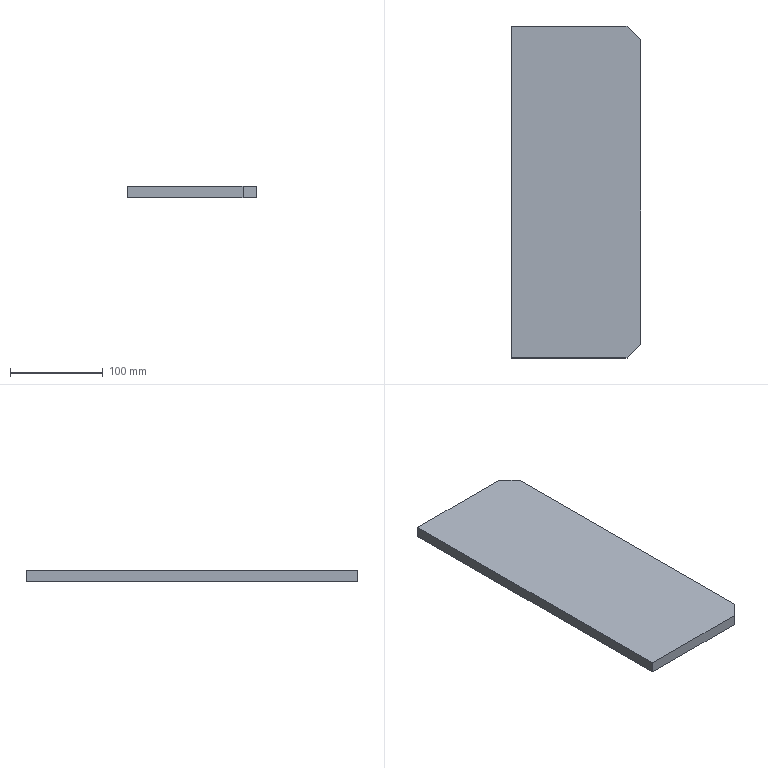Part | SolidWorks | features Chamfer 1, Extrusion 1 | 1 solid | 8 faces | box 140 x 358 x 12 mm | volume 598740 mm3 | plane 8
STEP:
#1=CARTESIAN_POINT('',(0.,358.,0.));
#2=VERTEX_POINT('',#1);
#3=CARTESIAN_POINT('',(0.,0.,0.));
#4=VERTEX_POINT('',#3);
#5=CARTESIAN_POINT('',(0.,0.,0.));
#6=DIRECTION('',(0.,-1.,0.));
#7=VECTOR('',#6,1000.);
#8=LINE('',#5,#7);
#9=EDGE_CURVE('',#2,#4,#8,.T.);
#10=ORIENTED_EDGE('',*,*,#9,.T.);
#11=CARTESIAN_POINT('',(0.,0.,12.));
#12=VERTEX_POINT('',#11);
#13=CARTESIAN_POINT('',(0.,0.,12.));
#14=DIRECTION('',(0.,0.,-1.));
#15=VECTOR('',#14,1000.);
#16=LINE('',#13,#15);
#17=EDGE_CURVE('',#12,#4,#16,.T.);
#18=ORIENTED_EDGE('',*,*,#17,.F.);
#19=CARTESIAN_POINT('',(0.,358.,12.));
#20=VERTEX_POINT('',#19);
#21=CARTESIAN_POINT('',(0.,0.,12.));
#22=DIRECTION('',(0.,-1.,0.));
#23=VECTOR('',#22,1000.);
#24=LINE('',#21,#23);
#25=EDGE_CURVE('',#20,#12,#24,.T.);
#26=ORIENTED_EDGE('',*,*,#25,.F.);
#27=CARTESIAN_POINT('',(0.,358.,12.));
#28=DIRECTION('',(0.,0.,-1.));
#29=VECTOR('',#28,1000.);
#30=LINE('',#27,#29);
#31=EDGE_CURVE('',#20,#2,#30,.T.);
#32=ORIENTED_EDGE('',*,*,#31,.T.);
#33=EDGE_LOOP('',(#10,#18,#26,#32));
#34=FACE_OUTER_BOUND('',#33,.T.);
#35=CARTESIAN_POINT('',(0.,0.,12.));
#36=DIRECTION('',(1.,0.,0.));
#37=DIRECTION('',(0.,0.,-1.));
#38=AXIS2_PLACEMENT_3D('',#35,#36,#37);
#39=PLANE('',#38);
#40=ADVANCED_FACE('',(#34),#39,.F.);
#41=CARTESIAN_POINT('',(125.,0.,0.));
#42=VERTEX_POINT('',#41);
#43=CARTESIAN_POINT('',(0.,0.,0.));
#44=DIRECTION('',(1.,0.,0.));
#45=VECTOR('',#44,1000.);
#46=LINE('',#43,#45);
#47=EDGE_CURVE('',#4,#42,#46,.T.);
#48=ORIENTED_EDGE('',*,*,#47,.T.);
#49=CARTESIAN_POINT('',(125.,0.,12.));
#50=VERTEX_POINT('',#49);
#51=CARTESIAN_POINT('',(125.,0.,12.));
#52=DIRECTION('',(0.,0.,1.));
#53=VECTOR('',#52,1000.);
#54=LINE('',#51,#53);
#55=EDGE_CURVE('',#42,#50,#54,.T.);
#56=ORIENTED_EDGE('',*,*,#55,.T.);
#57=CARTESIAN_POINT('',(0.,0.,12.));
#58=DIRECTION('',(1.,0.,0.));
#59=VECTOR('',#58,1000.);
#60=LINE('',#57,#59);
#61=EDGE_CURVE('',#12,#50,#60,.T.);
#62=ORIENTED_EDGE('',*,*,#61,.F.);
#63=ORIENTED_EDGE('',*,*,#17,.T.);
#64=EDGE_LOOP('',(#48,#56,#62,#63));
#65=FACE_OUTER_BOUND('',#64,.T.);
#66=CARTESIAN_POINT('',(0.,0.,12.));
#67=DIRECTION('',(0.,1.,0.));
#68=DIRECTION('',(0.,0.,1.));
#69=AXIS2_PLACEMENT_3D('',#66,#67,#68);
#70=PLANE('',#69);
#71=ADVANCED_FACE('',(#65),#70,.F.);
#72=CARTESIAN_POINT('',(140.,15.,12.));
#73=VERTEX_POINT('',#72);
#74=CARTESIAN_POINT('',(140.,343.,12.));
#75=VERTEX_POINT('',#74);
#76=CARTESIAN_POINT('',(140.,0.,12.));
#77=DIRECTION('',(0.,1.,0.));
#78=VECTOR('',#77,1000.);
#79=LINE('',#76,#78);
#80=EDGE_CURVE('',#73,#75,#79,.T.);
#81=ORIENTED_EDGE('',*,*,#80,.F.);
#82=CARTESIAN_POINT('',(140.,15.,0.));
#83=VERTEX_POINT('',#82);
#84=CARTESIAN_POINT('',(140.,15.,12.));
#85=DIRECTION('',(0.,0.,-1.));
#86=VECTOR('',#85,1000.);
#87=LINE('',#84,#86);
#88=EDGE_CURVE('',#73,#83,#87,.T.);
#89=ORIENTED_EDGE('',*,*,#88,.T.);
#90=CARTESIAN_POINT('',(140.,343.,0.));
#91=VERTEX_POINT('',#90);
#92=CARTESIAN_POINT('',(140.,0.,0.));
#93=DIRECTION('',(0.,1.,0.));
#94=VECTOR('',#93,1000.);
#95=LINE('',#92,#94);
#96=EDGE_CURVE('',#83,#91,#95,.T.);
#97=ORIENTED_EDGE('',*,*,#96,.T.);
#98=CARTESIAN_POINT('',(140.,343.,12.));
#99=DIRECTION('',(0.,0.,1.));
#100=VECTOR('',#99,1000.);
#101=LINE('',#98,#100);
#102=EDGE_CURVE('',#91,#75,#101,.T.);
#103=ORIENTED_EDGE('',*,*,#102,.T.);
#104=EDGE_LOOP('',(#81,#89,#97,#103));
#105=FACE_OUTER_BOUND('',#104,.T.);
#106=CARTESIAN_POINT('',(140.,0.,12.));
#107=DIRECTION('',(-1.,0.,0.));
#108=DIRECTION('',(0.,0.,1.));
#109=AXIS2_PLACEMENT_3D('',#106,#107,#108);
#110=PLANE('',#109);
#111=ADVANCED_FACE('',(#105),#110,.F.);
#112=CARTESIAN_POINT('',(125.,358.,12.));
#113=VERTEX_POINT('',#112);
#114=CARTESIAN_POINT('',(0.,358.,12.));
#115=DIRECTION('',(-1.,0.,0.));
#116=VECTOR('',#115,1000.);
#117=LINE('',#114,#116);
#118=EDGE_CURVE('',#113,#20,#117,.T.);
#119=ORIENTED_EDGE('',*,*,#118,.F.);
#120=CARTESIAN_POINT('',(125.,358.,0.));
#121=VERTEX_POINT('',#120);
#122=CARTESIAN_POINT('',(125.,358.,12.));
#123=DIRECTION('',(0.,0.,-1.));
#124=VECTOR('',#123,1000.);
#125=LINE('',#122,#124);
#126=EDGE_CURVE('',#113,#121,#125,.T.);
#127=ORIENTED_EDGE('',*,*,#126,.T.);
#128=CARTESIAN_POINT('',(0.,358.,0.));
#129=DIRECTION('',(-1.,0.,0.));
#130=VECTOR('',#129,1000.);
#131=LINE('',#128,#130);
#132=EDGE_CURVE('',#121,#2,#131,.T.);
#133=ORIENTED_EDGE('',*,*,#132,.T.);
#134=ORIENTED_EDGE('',*,*,#31,.F.);
#135=EDGE_LOOP('',(#119,#127,#133,#134));
#136=FACE_OUTER_BOUND('',#135,.T.);
#137=CARTESIAN_POINT('',(0.,358.,12.));
#138=DIRECTION('',(0.,-1.,0.));
#139=DIRECTION('',(0.,0.,-1.));
#140=AXIS2_PLACEMENT_3D('',#137,#138,#139);
#141=PLANE('',#140);
#142=ADVANCED_FACE('',(#136),#141,.F.);
#143=ORIENTED_EDGE('',*,*,#61,.T.);
#144=CARTESIAN_POINT('',(140.,15.,12.));
#145=DIRECTION('',(0.7071,0.7071,0.));
#146=VECTOR('',#145,1000.);
#147=LINE('',#144,#146);
#148=EDGE_CURVE('',#50,#73,#147,.T.);
#149=ORIENTED_EDGE('',*,*,#148,.T.);
#150=ORIENTED_EDGE('',*,*,#80,.T.);
#151=CARTESIAN_POINT('',(125.,358.,12.));
#152=DIRECTION('',(-0.7071,0.7071,0.));
#153=VECTOR('',#152,1000.);
#154=LINE('',#151,#153);
#155=EDGE_CURVE('',#75,#113,#154,.T.);
#156=ORIENTED_EDGE('',*,*,#155,.T.);
#157=ORIENTED_EDGE('',*,*,#118,.T.);
#158=ORIENTED_EDGE('',*,*,#25,.T.);
#159=EDGE_LOOP('',(#143,#149,#150,#156,#157,#158));
#160=FACE_OUTER_BOUND('',#159,.T.);
#161=CARTESIAN_POINT('',(0.,0.,12.));
#162=DIRECTION('',(0.,0.,-1.));
#163=DIRECTION('',(-1.,0.,0.));
#164=AXIS2_PLACEMENT_3D('',#161,#162,#163);
#165=PLANE('',#164);
#166=ADVANCED_FACE('',(#160),#165,.F.);
#167=ORIENTED_EDGE('',*,*,#96,.F.);
#168=CARTESIAN_POINT('',(62.5,-62.5,0.));
#169=DIRECTION('',(-0.7071,-0.7071,0.));
#170=VECTOR('',#169,1000.);
#171=LINE('',#168,#170);
#172=EDGE_CURVE('',#83,#42,#171,.T.);
#173=ORIENTED_EDGE('',*,*,#172,.T.);
#174=ORIENTED_EDGE('',*,*,#47,.F.);
#175=ORIENTED_EDGE('',*,*,#9,.F.);
#176=ORIENTED_EDGE('',*,*,#132,.F.);
#177=CARTESIAN_POINT('',(241.5,241.5,0.));
#178=DIRECTION('',(0.7071,-0.7071,0.));
#179=VECTOR('',#178,1000.);
#180=LINE('',#177,#179);
#181=EDGE_CURVE('',#121,#91,#180,.T.);
#182=ORIENTED_EDGE('',*,*,#181,.T.);
#183=EDGE_LOOP('',(#167,#173,#174,#175,#176,#182));
#184=FACE_OUTER_BOUND('',#183,.T.);
#185=CARTESIAN_POINT('',(0.,0.,0.));
#186=DIRECTION('',(0.,0.,-1.));
#187=DIRECTION('',(-1.,0.,0.));
#188=AXIS2_PLACEMENT_3D('',#185,#186,#187);
#189=PLANE('',#188);
#190=ADVANCED_FACE('',(#184),#189,.T.);
#191=ORIENTED_EDGE('',*,*,#148,.F.);
#192=ORIENTED_EDGE('',*,*,#55,.F.);
#193=ORIENTED_EDGE('',*,*,#172,.F.);
#194=ORIENTED_EDGE('',*,*,#88,.F.);
#195=EDGE_LOOP('',(#191,#192,#193,#194));
#196=FACE_OUTER_BOUND('',#195,.T.);
#197=CARTESIAN_POINT('',(140.,15.,12.));
#198=DIRECTION('',(-0.7071,0.7071,0.));
#199=DIRECTION('',(0.,0.,-1.));
#200=AXIS2_PLACEMENT_3D('',#197,#198,#199);
#201=PLANE('',#200);
#202=ADVANCED_FACE('',(#196),#201,.F.);
#203=ORIENTED_EDGE('',*,*,#155,.F.);
#204=ORIENTED_EDGE('',*,*,#102,.F.);
#205=ORIENTED_EDGE('',*,*,#181,.F.);
#206=ORIENTED_EDGE('',*,*,#126,.F.);
#207=EDGE_LOOP('',(#203,#204,#205,#206));
#208=FACE_OUTER_BOUND('',#207,.T.);
#209=CARTESIAN_POINT('',(125.,358.,12.));
#210=DIRECTION('',(-0.7071,-0.7071,0.));
#211=DIRECTION('',(0.,0.,-1.));
#212=AXIS2_PLACEMENT_3D('',#209,#210,#211);
#213=PLANE('',#212);
#214=ADVANCED_FACE('',(#208),#213,.F.);
#215=CLOSED_SHELL('',(#40,#71,#111,#142,#166,#190,#202,#214));
#216=MANIFOLD_SOLID_BREP('',#215);
#217=CARTESIAN_POINT('',(0.,0.,0.));
#218=DIRECTION('',(0.,0.,1.));
#219=DIRECTION('',(1.,0.,0.));
#220=AXIS2_PLACEMENT_3D('',#217,#218,#219);
#221=(LENGTH_UNIT()NAMED_UNIT(*)SI_UNIT(.MILLI.,.METRE.));
#222=UNCERTAINTY_MEASURE_WITH_UNIT(LENGTH_MEASURE(0.00001),#221,'','');
#223=(NAMED_UNIT(*)PLANE_ANGLE_UNIT()SI_UNIT($,.RADIAN.));
#224=(NAMED_UNIT(*)SI_UNIT($,.STERADIAN.)SOLID_ANGLE_UNIT());
#225=(GEOMETRIC_REPRESENTATION_CONTEXT(3)GLOBAL_UNCERTAINTY_ASSIGNED_CONTEXT((#222))GLOBAL_UNIT_ASSIGNED_CONTEXT((#221,#223,#224))REPRESENTATION_CONTEXT('',''));
#226=ADVANCED_BREP_SHAPE_REPRESENTATION('',(#216,#220),#225);